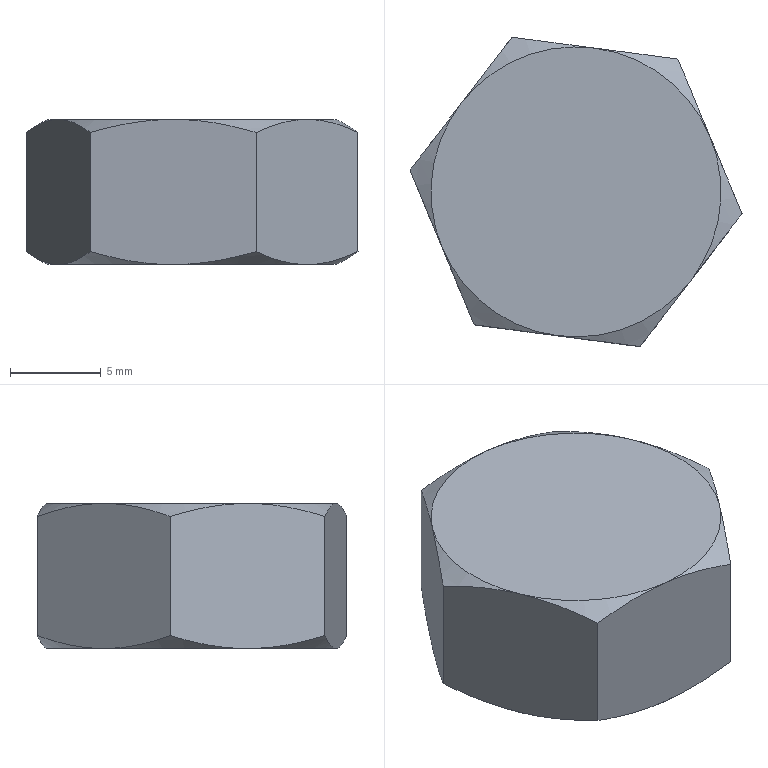Part | SolidWorks | features BaseBody 1 | 1 solid | 20 faces | box 18.318 x 17.066 x 8 mm | volume 1765 mm3 | cone 12 | plane 8
STEP:
#1=CARTESIAN_POINT('',(-45.504,-13.036,-254.55));
#2=VERTEX_POINT('',#1);
#3=CARTESIAN_POINT('',(-51.853,-8.168,-254.55));
#4=VERTEX_POINT('',#3);
#5=CARTESIAN_POINT('',(-44.463,-5.104,-254.55));
#6=DIRECTION('',(0.,0.,-1.));
#7=DIRECTION('',(-0.9237,-0.383,0.));
#8=AXIS2_PLACEMENT_3D('',#5,#6,#7);
#9=CIRCLE('',#8,8.);
#10=EDGE_CURVE('',#2,#4,#9,.T.);
#11=ORIENTED_EDGE('',*,*,#10,.T.);
#12=CARTESIAN_POINT('',(-50.812,-0.2362,-254.55));
#13=VERTEX_POINT('',#12);
#14=CARTESIAN_POINT('',(-44.463,-5.104,-254.55));
#15=DIRECTION('',(0.,0.,-1.));
#16=DIRECTION('',(-0.9237,-0.383,0.));
#17=AXIS2_PLACEMENT_3D('',#14,#15,#16);
#18=CIRCLE('',#17,8.);
#19=EDGE_CURVE('',#4,#13,#18,.T.);
#20=ORIENTED_EDGE('',*,*,#19,.T.);
#21=CARTESIAN_POINT('',(-43.422,2.828,-254.55));
#22=VERTEX_POINT('',#21);
#23=CARTESIAN_POINT('',(-44.463,-5.104,-254.55));
#24=DIRECTION('',(0.,0.,-1.));
#25=DIRECTION('',(-0.9237,-0.383,0.));
#26=AXIS2_PLACEMENT_3D('',#23,#24,#25);
#27=CIRCLE('',#26,8.);
#28=EDGE_CURVE('',#13,#22,#27,.T.);
#29=ORIENTED_EDGE('',*,*,#28,.T.);
#30=CARTESIAN_POINT('',(-37.073,-2.039,-254.55));
#31=VERTEX_POINT('',#30);
#32=CARTESIAN_POINT('',(-44.463,-5.104,-254.55));
#33=DIRECTION('',(0.,0.,1.));
#34=DIRECTION('',(0.9237,0.383,0.));
#35=AXIS2_PLACEMENT_3D('',#32,#33,#34);
#36=CIRCLE('',#35,8.);
#37=EDGE_CURVE('',#31,#22,#36,.T.);
#38=ORIENTED_EDGE('',*,*,#37,.F.);
#39=CARTESIAN_POINT('',(-38.114,-9.971,-254.55));
#40=VERTEX_POINT('',#39);
#41=CARTESIAN_POINT('',(-44.463,-5.104,-254.55));
#42=DIRECTION('',(0.,0.,-1.));
#43=DIRECTION('',(-0.9237,-0.383,0.));
#44=AXIS2_PLACEMENT_3D('',#41,#42,#43);
#45=CIRCLE('',#44,8.);
#46=EDGE_CURVE('',#31,#40,#45,.T.);
#47=ORIENTED_EDGE('',*,*,#46,.T.);
#48=CARTESIAN_POINT('',(-44.463,-5.104,-254.55));
#49=DIRECTION('',(0.,0.,-1.));
#50=DIRECTION('',(-0.9237,-0.383,0.));
#51=AXIS2_PLACEMENT_3D('',#48,#49,#50);
#52=CIRCLE('',#51,8.);
#53=EDGE_CURVE('',#40,#2,#52,.T.);
#54=ORIENTED_EDGE('',*,*,#53,.T.);
#55=EDGE_LOOP('',(#11,#20,#29,#38,#47,#54));
#56=FACE_OUTER_BOUND('',#55,.T.);
#57=CARTESIAN_POINT('',(-42.381,10.76,-254.55));
#58=DIRECTION('',(0.,0.,-1.));
#59=DIRECTION('',(0.,-1.,0.));
#60=AXIS2_PLACEMENT_3D('',#57,#58,#59);
#61=PLANE('',#60);
#62=ADVANCED_FACE('',(#56),#61,.T.);
#63=CARTESIAN_POINT('',(-53.622,-3.902,-253.835));
#64=VERTEX_POINT('',#63);
#65=CARTESIAN_POINT('',(-53.622,-3.902,-253.835));
#66=CARTESIAN_POINT('',(-53.163,-3.303,-254.053));
#67=CARTESIAN_POINT('',(-52.7,-2.699,-254.233));
#68=CARTESIAN_POINT('',(-51.764,-1.479,-254.482));
#69=CARTESIAN_POINT('',(-51.291,-0.8617,-254.55));
#70=CARTESIAN_POINT('',(-50.812,-0.2362,-254.55));
#71=B_SPLINE_CURVE_WITH_KNOTS('',3,(#65,#66,#67,#68,#69,#70),.UNSPECIFIED.,.F.,.F.,(4,2,4),(0.,0.002337,0.004674),.UNSPECIFIED.);
#72=EDGE_CURVE('',#64,#13,#71,.T.);
#73=ORIENTED_EDGE('',*,*,#72,.T.);
#74=ORIENTED_EDGE('',*,*,#19,.F.);
#75=CARTESIAN_POINT('',(-51.853,-8.168,-254.55));
#76=CARTESIAN_POINT('',(-52.155,-7.44,-254.55));
#77=CARTESIAN_POINT('',(-52.453,-6.722,-254.482));
#78=CARTESIAN_POINT('',(-53.042,-5.301,-254.233));
#79=CARTESIAN_POINT('',(-53.333,-4.599,-254.053));
#80=CARTESIAN_POINT('',(-53.622,-3.902,-253.835));
#81=B_SPLINE_CURVE_WITH_KNOTS('',3,(#75,#76,#77,#78,#79,#80),.UNSPECIFIED.,.F.,.F.,(4,2,4),(0.,0.002337,0.004674),.UNSPECIFIED.);
#82=EDGE_CURVE('',#4,#64,#81,.T.);
#83=ORIENTED_EDGE('',*,*,#82,.T.);
#84=EDGE_LOOP('',(#73,#74,#83));
#85=FACE_OUTER_BOUND('',#84,.T.);
#86=CARTESIAN_POINT('',(-44.463,-5.104,-251.646));
#87=DIRECTION('',(0.,0.,1.));
#88=DIRECTION('',(0.9237,0.383,0.));
#89=AXIS2_PLACEMENT_3D('',#86,#87,#88);
#90=CONICAL_SURFACE('',#89,13.029,1.047);
#91=ADVANCED_FACE('',(#85),#90,.T.);
#92=CARTESIAN_POINT('',(-48.001,3.429,-253.835));
#93=VERTEX_POINT('',#92);
#94=CARTESIAN_POINT('',(-50.812,-0.2362,-254.55));
#95=CARTESIAN_POINT('',(-50.332,0.3893,-254.55));
#96=CARTESIAN_POINT('',(-49.859,1.006,-254.482));
#97=CARTESIAN_POINT('',(-48.923,2.227,-254.233));
#98=CARTESIAN_POINT('',(-48.46,2.83,-254.053));
#99=CARTESIAN_POINT('',(-48.001,3.429,-253.835));
#100=B_SPLINE_CURVE_WITH_KNOTS('',3,(#94,#95,#96,#97,#98,#99),.UNSPECIFIED.,.F.,.F.,(4,2,4),(0.,0.002337,0.004674),.UNSPECIFIED.);
#101=EDGE_CURVE('',#13,#93,#100,.T.);
#102=ORIENTED_EDGE('',*,*,#101,.T.);
#103=CARTESIAN_POINT('',(-48.001,3.429,-253.835));
#104=CARTESIAN_POINT('',(-47.253,3.331,-254.053));
#105=CARTESIAN_POINT('',(-46.499,3.232,-254.233));
#106=CARTESIAN_POINT('',(-44.974,3.032,-254.482));
#107=CARTESIAN_POINT('',(-44.203,2.931,-254.55));
#108=CARTESIAN_POINT('',(-43.422,2.828,-254.55));
#109=B_SPLINE_CURVE_WITH_KNOTS('',3,(#103,#104,#105,#106,#107,#108),.UNSPECIFIED.,.F.,.F.,(4,2,4),(0.,0.002337,0.004674),.UNSPECIFIED.);
#110=EDGE_CURVE('',#93,#22,#109,.T.);
#111=ORIENTED_EDGE('',*,*,#110,.T.);
#112=ORIENTED_EDGE('',*,*,#28,.F.);
#113=EDGE_LOOP('',(#102,#111,#112));
#114=FACE_OUTER_BOUND('',#113,.T.);
#115=CARTESIAN_POINT('',(-44.463,-5.104,-251.646));
#116=DIRECTION('',(0.,0.,1.));
#117=DIRECTION('',(0.9237,0.383,0.));
#118=AXIS2_PLACEMENT_3D('',#115,#116,#117);
#119=CONICAL_SURFACE('',#118,13.029,1.047);
#120=ADVANCED_FACE('',(#114),#119,.T.);
#121=CARTESIAN_POINT('',(-38.842,2.227,-253.835));
#122=VERTEX_POINT('',#121);
#123=CARTESIAN_POINT('',(-43.422,2.828,-254.55));
#124=CARTESIAN_POINT('',(-42.64,2.726,-254.55));
#125=CARTESIAN_POINT('',(-41.869,2.624,-254.482));
#126=CARTESIAN_POINT('',(-40.344,2.424,-254.233));
#127=CARTESIAN_POINT('',(-39.59,2.325,-254.053));
#128=CARTESIAN_POINT('',(-38.842,2.227,-253.835));
#129=B_SPLINE_CURVE_WITH_KNOTS('',3,(#123,#124,#125,#126,#127,#128),.UNSPECIFIED.,.F.,.F.,(4,2,4),(0.,0.002337,0.004674),.UNSPECIFIED.);
#130=EDGE_CURVE('',#22,#122,#129,.T.);
#131=ORIENTED_EDGE('',*,*,#130,.T.);
#132=CARTESIAN_POINT('',(-38.842,2.227,-253.835));
#133=CARTESIAN_POINT('',(-38.553,1.53,-254.053));
#134=CARTESIAN_POINT('',(-38.262,0.8277,-254.233));
#135=CARTESIAN_POINT('',(-37.673,-0.5929,-254.482));
#136=CARTESIAN_POINT('',(-37.375,-1.311,-254.55));
#137=CARTESIAN_POINT('',(-37.073,-2.039,-254.55));
#138=B_SPLINE_CURVE_WITH_KNOTS('',3,(#132,#133,#134,#135,#136,#137),.UNSPECIFIED.,.F.,.F.,(4,2,4),(0.,0.002337,0.004674),.UNSPECIFIED.);
#139=EDGE_CURVE('',#122,#31,#138,.T.);
#140=ORIENTED_EDGE('',*,*,#139,.T.);
#141=ORIENTED_EDGE('',*,*,#37,.T.);
#142=EDGE_LOOP('',(#131,#140,#141));
#143=FACE_OUTER_BOUND('',#142,.T.);
#144=CARTESIAN_POINT('',(-44.463,-5.104,-251.646));
#145=DIRECTION('',(0.,0.,1.));
#146=DIRECTION('',(0.9237,0.383,0.));
#147=AXIS2_PLACEMENT_3D('',#144,#145,#146);
#148=CONICAL_SURFACE('',#147,13.029,1.047);
#149=ADVANCED_FACE('',(#143),#148,.T.);
#150=CARTESIAN_POINT('',(-35.304,-6.306,-253.835));
#151=VERTEX_POINT('',#150);
#152=CARTESIAN_POINT('',(-37.073,-2.039,-254.55));
#153=CARTESIAN_POINT('',(-36.771,-2.767,-254.55));
#154=CARTESIAN_POINT('',(-36.473,-3.486,-254.482));
#155=CARTESIAN_POINT('',(-35.884,-4.906,-254.233));
#156=CARTESIAN_POINT('',(-35.593,-5.609,-254.053));
#157=CARTESIAN_POINT('',(-35.304,-6.306,-253.835));
#158=B_SPLINE_CURVE_WITH_KNOTS('',3,(#152,#153,#154,#155,#156,#157),.UNSPECIFIED.,.F.,.F.,(4,2,4),(0.,0.002337,0.004674),.UNSPECIFIED.);
#159=EDGE_CURVE('',#31,#151,#158,.T.);
#160=ORIENTED_EDGE('',*,*,#159,.T.);
#161=CARTESIAN_POINT('',(-35.304,-6.306,-253.835));
#162=CARTESIAN_POINT('',(-35.763,-6.905,-254.053));
#163=CARTESIAN_POINT('',(-36.226,-7.508,-254.233));
#164=CARTESIAN_POINT('',(-37.161,-8.729,-254.482));
#165=CARTESIAN_POINT('',(-37.635,-9.346,-254.55));
#166=CARTESIAN_POINT('',(-38.114,-9.971,-254.55));
#167=B_SPLINE_CURVE_WITH_KNOTS('',3,(#161,#162,#163,#164,#165,#166),.UNSPECIFIED.,.F.,.F.,(4,2,4),(0.,0.002337,0.004674),.UNSPECIFIED.);
#168=EDGE_CURVE('',#151,#40,#167,.T.);
#169=ORIENTED_EDGE('',*,*,#168,.T.);
#170=ORIENTED_EDGE('',*,*,#46,.F.);
#171=EDGE_LOOP('',(#160,#169,#170));
#172=FACE_OUTER_BOUND('',#171,.T.);
#173=CARTESIAN_POINT('',(-44.463,-5.104,-251.646));
#174=DIRECTION('',(0.,0.,1.));
#175=DIRECTION('',(0.9237,0.383,0.));
#176=AXIS2_PLACEMENT_3D('',#173,#174,#175);
#177=CONICAL_SURFACE('',#176,13.029,1.047);
#178=ADVANCED_FACE('',(#172),#177,.T.);
#179=CARTESIAN_POINT('',(-40.924,-13.637,-253.835));
#180=VERTEX_POINT('',#179);
#181=CARTESIAN_POINT('',(-38.114,-9.971,-254.55));
#182=CARTESIAN_POINT('',(-38.594,-10.597,-254.55));
#183=CARTESIAN_POINT('',(-39.067,-11.214,-254.482));
#184=CARTESIAN_POINT('',(-40.003,-12.435,-254.233));
#185=CARTESIAN_POINT('',(-40.465,-13.038,-254.053));
#186=CARTESIAN_POINT('',(-40.924,-13.637,-253.835));
#187=B_SPLINE_CURVE_WITH_KNOTS('',3,(#181,#182,#183,#184,#185,#186),.UNSPECIFIED.,.F.,.F.,(4,2,4),(0.,0.002337,0.004674),.UNSPECIFIED.);
#188=EDGE_CURVE('',#40,#180,#187,.T.);
#189=ORIENTED_EDGE('',*,*,#188,.T.);
#190=CARTESIAN_POINT('',(-40.924,-13.637,-253.835));
#191=CARTESIAN_POINT('',(-41.673,-13.539,-254.053));
#192=CARTESIAN_POINT('',(-42.426,-13.44,-254.233));
#193=CARTESIAN_POINT('',(-43.951,-13.24,-254.482));
#194=CARTESIAN_POINT('',(-44.722,-13.138,-254.55));
#195=CARTESIAN_POINT('',(-45.504,-13.036,-254.55));
#196=B_SPLINE_CURVE_WITH_KNOTS('',3,(#190,#191,#192,#193,#194,#195),.UNSPECIFIED.,.F.,.F.,(4,2,4),(0.,0.002337,0.004674),.UNSPECIFIED.);
#197=EDGE_CURVE('',#180,#2,#196,.T.);
#198=ORIENTED_EDGE('',*,*,#197,.T.);
#199=ORIENTED_EDGE('',*,*,#53,.F.);
#200=EDGE_LOOP('',(#189,#198,#199));
#201=FACE_OUTER_BOUND('',#200,.T.);
#202=CARTESIAN_POINT('',(-44.463,-5.104,-251.646));
#203=DIRECTION('',(0.,0.,1.));
#204=DIRECTION('',(0.9237,0.383,0.));
#205=AXIS2_PLACEMENT_3D('',#202,#203,#204);
#206=CONICAL_SURFACE('',#205,13.029,1.047);
#207=ADVANCED_FACE('',(#201),#206,.T.);
#208=CARTESIAN_POINT('',(-50.083,-12.435,-253.835));
#209=VERTEX_POINT('',#208);
#210=CARTESIAN_POINT('',(-45.504,-13.036,-254.55));
#211=CARTESIAN_POINT('',(-46.285,-12.933,-254.55));
#212=CARTESIAN_POINT('',(-47.057,-12.832,-254.482));
#213=CARTESIAN_POINT('',(-48.581,-12.632,-254.233));
#214=CARTESIAN_POINT('',(-49.335,-12.533,-254.053));
#215=CARTESIAN_POINT('',(-50.083,-12.435,-253.835));
#216=B_SPLINE_CURVE_WITH_KNOTS('',3,(#210,#211,#212,#213,#214,#215),.UNSPECIFIED.,.F.,.F.,(4,2,4),(0.,0.002337,0.004674),.UNSPECIFIED.);
#217=EDGE_CURVE('',#2,#209,#216,.T.);
#218=ORIENTED_EDGE('',*,*,#217,.T.);
#219=CARTESIAN_POINT('',(-50.083,-12.435,-253.835));
#220=CARTESIAN_POINT('',(-50.372,-11.738,-254.053));
#221=CARTESIAN_POINT('',(-50.664,-11.035,-254.233));
#222=CARTESIAN_POINT('',(-51.253,-9.615,-254.482));
#223=CARTESIAN_POINT('',(-51.551,-8.896,-254.55));
#224=CARTESIAN_POINT('',(-51.853,-8.168,-254.55));
#225=B_SPLINE_CURVE_WITH_KNOTS('',3,(#219,#220,#221,#222,#223,#224),.UNSPECIFIED.,.F.,.F.,(4,2,4),(0.,0.002337,0.004674),.UNSPECIFIED.);
#226=EDGE_CURVE('',#209,#4,#225,.T.);
#227=ORIENTED_EDGE('',*,*,#226,.T.);
#228=ORIENTED_EDGE('',*,*,#10,.F.);
#229=EDGE_LOOP('',(#218,#227,#228));
#230=FACE_OUTER_BOUND('',#229,.T.);
#231=CARTESIAN_POINT('',(-44.463,-5.104,-251.646));
#232=DIRECTION('',(0.,0.,1.));
#233=DIRECTION('',(0.9237,0.383,0.));
#234=AXIS2_PLACEMENT_3D('',#231,#232,#233);
#235=CONICAL_SURFACE('',#234,13.029,1.047);
#236=ADVANCED_FACE('',(#230),#235,.T.);
#237=CARTESIAN_POINT('',(-51.853,-8.168,-246.55));
#238=VERTEX_POINT('',#237);
#239=CARTESIAN_POINT('',(-50.812,-0.2362,-246.55));
#240=VERTEX_POINT('',#239);
#241=CARTESIAN_POINT('',(-44.463,-5.104,-246.55));
#242=DIRECTION('',(0.,0.,-1.));
#243=DIRECTION('',(-0.9237,-0.383,0.));
#244=AXIS2_PLACEMENT_3D('',#241,#242,#243);
#245=CIRCLE('',#244,8.);
#246=EDGE_CURVE('',#238,#240,#245,.T.);
#247=ORIENTED_EDGE('',*,*,#246,.F.);
#248=CARTESIAN_POINT('',(-45.504,-13.036,-246.55));
#249=VERTEX_POINT('',#248);
#250=CARTESIAN_POINT('',(-44.463,-5.104,-246.55));
#251=DIRECTION('',(0.,0.,-1.));
#252=DIRECTION('',(-0.9237,-0.383,0.));
#253=AXIS2_PLACEMENT_3D('',#250,#251,#252);
#254=CIRCLE('',#253,8.);
#255=EDGE_CURVE('',#249,#238,#254,.T.);
#256=ORIENTED_EDGE('',*,*,#255,.F.);
#257=CARTESIAN_POINT('',(-38.114,-9.971,-246.55));
#258=VERTEX_POINT('',#257);
#259=CARTESIAN_POINT('',(-44.463,-5.104,-246.55));
#260=DIRECTION('',(0.,0.,-1.));
#261=DIRECTION('',(-0.9237,-0.383,0.));
#262=AXIS2_PLACEMENT_3D('',#259,#260,#261);
#263=CIRCLE('',#262,8.);
#264=EDGE_CURVE('',#258,#249,#263,.T.);
#265=ORIENTED_EDGE('',*,*,#264,.F.);
#266=CARTESIAN_POINT('',(-37.073,-2.039,-246.55));
#267=VERTEX_POINT('',#266);
#268=CARTESIAN_POINT('',(-44.463,-5.104,-246.55));
#269=DIRECTION('',(0.,0.,-1.));
#270=DIRECTION('',(-0.9237,-0.383,0.));
#271=AXIS2_PLACEMENT_3D('',#268,#269,#270);
#272=CIRCLE('',#271,8.);
#273=EDGE_CURVE('',#267,#258,#272,.T.);
#274=ORIENTED_EDGE('',*,*,#273,.F.);
#275=CARTESIAN_POINT('',(-43.422,2.828,-246.55));
#276=VERTEX_POINT('',#275);
#277=CARTESIAN_POINT('',(-44.463,-5.104,-246.55));
#278=DIRECTION('',(0.,0.,1.));
#279=DIRECTION('',(0.9237,0.383,0.));
#280=AXIS2_PLACEMENT_3D('',#277,#278,#279);
#281=CIRCLE('',#280,8.);
#282=EDGE_CURVE('',#267,#276,#281,.T.);
#283=ORIENTED_EDGE('',*,*,#282,.T.);
#284=CARTESIAN_POINT('',(-44.463,-5.104,-246.55));
#285=DIRECTION('',(0.,0.,-1.));
#286=DIRECTION('',(-0.9237,-0.383,0.));
#287=AXIS2_PLACEMENT_3D('',#284,#285,#286);
#288=CIRCLE('',#287,8.);
#289=EDGE_CURVE('',#240,#276,#288,.T.);
#290=ORIENTED_EDGE('',*,*,#289,.F.);
#291=EDGE_LOOP('',(#247,#256,#265,#274,#283,#290));
#292=FACE_OUTER_BOUND('',#291,.T.);
#293=CARTESIAN_POINT('',(-42.381,10.76,-246.55));
#294=DIRECTION('',(0.,0.,-1.));
#295=DIRECTION('',(0.,-1.,0.));
#296=AXIS2_PLACEMENT_3D('',#293,#294,#295);
#297=PLANE('',#296);
#298=ADVANCED_FACE('',(#292),#297,.F.);
#299=CARTESIAN_POINT('',(-53.622,-3.902,-247.265));
#300=VERTEX_POINT('',#299);
#301=CARTESIAN_POINT('',(-50.812,-0.2362,-246.55));
#302=CARTESIAN_POINT('',(-51.291,-0.8617,-246.55));
#303=CARTESIAN_POINT('',(-51.764,-1.479,-246.618));
#304=CARTESIAN_POINT('',(-52.7,-2.699,-246.867));
#305=CARTESIAN_POINT('',(-53.163,-3.303,-247.047));
#306=CARTESIAN_POINT('',(-53.622,-3.902,-247.265));
#307=B_SPLINE_CURVE_WITH_KNOTS('',3,(#301,#302,#303,#304,#305,#306),.UNSPECIFIED.,.F.,.F.,(4,2,4),(0.,0.002337,0.004674),.UNSPECIFIED.);
#308=EDGE_CURVE('',#240,#300,#307,.T.);
#309=ORIENTED_EDGE('',*,*,#308,.T.);
#310=CARTESIAN_POINT('',(-53.622,-3.902,-247.265));
#311=CARTESIAN_POINT('',(-53.333,-4.599,-247.047));
#312=CARTESIAN_POINT('',(-53.042,-5.301,-246.867));
#313=CARTESIAN_POINT('',(-52.453,-6.722,-246.618));
#314=CARTESIAN_POINT('',(-52.155,-7.44,-246.55));
#315=CARTESIAN_POINT('',(-51.853,-8.168,-246.55));
#316=B_SPLINE_CURVE_WITH_KNOTS('',3,(#310,#311,#312,#313,#314,#315),.UNSPECIFIED.,.F.,.F.,(4,2,4),(0.,0.002337,0.004674),.UNSPECIFIED.);
#317=EDGE_CURVE('',#300,#238,#316,.T.);
#318=ORIENTED_EDGE('',*,*,#317,.T.);
#319=ORIENTED_EDGE('',*,*,#246,.T.);
#320=EDGE_LOOP('',(#309,#318,#319));
#321=FACE_OUTER_BOUND('',#320,.T.);
#322=CARTESIAN_POINT('',(-44.463,-5.104,-246.55));
#323=DIRECTION('',(0.,0.,-1.));
#324=DIRECTION('',(-0.9237,-0.383,0.));
#325=AXIS2_PLACEMENT_3D('',#322,#323,#324);
#326=CONICAL_SURFACE('',#325,8.,1.047);
#327=ADVANCED_FACE('',(#321),#326,.T.);
#328=CARTESIAN_POINT('',(-48.001,3.429,-247.265));
#329=VERTEX_POINT('',#328);
#330=CARTESIAN_POINT('',(-43.422,2.828,-246.55));
#331=CARTESIAN_POINT('',(-44.203,2.931,-246.55));
#332=CARTESIAN_POINT('',(-44.974,3.032,-246.618));
#333=CARTESIAN_POINT('',(-46.499,3.232,-246.867));
#334=CARTESIAN_POINT('',(-47.253,3.331,-247.047));
#335=CARTESIAN_POINT('',(-48.001,3.429,-247.265));
#336=B_SPLINE_CURVE_WITH_KNOTS('',3,(#330,#331,#332,#333,#334,#335),.UNSPECIFIED.,.F.,.F.,(4,2,4),(0.,0.002337,0.004674),.UNSPECIFIED.);
#337=EDGE_CURVE('',#276,#329,#336,.T.);
#338=ORIENTED_EDGE('',*,*,#337,.T.);
#339=CARTESIAN_POINT('',(-48.001,3.429,-247.265));
#340=CARTESIAN_POINT('',(-48.46,2.83,-247.047));
#341=CARTESIAN_POINT('',(-48.923,2.227,-246.867));
#342=CARTESIAN_POINT('',(-49.859,1.006,-246.618));
#343=CARTESIAN_POINT('',(-50.332,0.3893,-246.55));
#344=CARTESIAN_POINT('',(-50.812,-0.2362,-246.55));
#345=B_SPLINE_CURVE_WITH_KNOTS('',3,(#339,#340,#341,#342,#343,#344),.UNSPECIFIED.,.F.,.F.,(4,2,4),(0.,0.002337,0.004674),.UNSPECIFIED.);
#346=EDGE_CURVE('',#329,#240,#345,.T.);
#347=ORIENTED_EDGE('',*,*,#346,.T.);
#348=ORIENTED_EDGE('',*,*,#289,.T.);
#349=EDGE_LOOP('',(#338,#347,#348));
#350=FACE_OUTER_BOUND('',#349,.T.);
#351=CARTESIAN_POINT('',(-44.463,-5.104,-246.55));
#352=DIRECTION('',(0.,0.,-1.));
#353=DIRECTION('',(-0.9237,-0.383,0.));
#354=AXIS2_PLACEMENT_3D('',#351,#352,#353);
#355=CONICAL_SURFACE('',#354,8.,1.047);
#356=ADVANCED_FACE('',(#350),#355,.T.);
#357=CARTESIAN_POINT('',(-38.842,2.227,-247.265));
#358=VERTEX_POINT('',#357);
#359=CARTESIAN_POINT('',(-37.073,-2.039,-246.55));
#360=CARTESIAN_POINT('',(-37.375,-1.311,-246.55));
#361=CARTESIAN_POINT('',(-37.673,-0.5929,-246.618));
#362=CARTESIAN_POINT('',(-38.262,0.8277,-246.867));
#363=CARTESIAN_POINT('',(-38.553,1.53,-247.047));
#364=CARTESIAN_POINT('',(-38.842,2.227,-247.265));
#365=B_SPLINE_CURVE_WITH_KNOTS('',3,(#359,#360,#361,#362,#363,#364),.UNSPECIFIED.,.F.,.F.,(4,2,4),(0.,0.002337,0.004674),.UNSPECIFIED.);
#366=EDGE_CURVE('',#267,#358,#365,.T.);
#367=ORIENTED_EDGE('',*,*,#366,.T.);
#368=CARTESIAN_POINT('',(-38.842,2.227,-247.265));
#369=CARTESIAN_POINT('',(-39.59,2.325,-247.047));
#370=CARTESIAN_POINT('',(-40.344,2.424,-246.867));
#371=CARTESIAN_POINT('',(-41.869,2.624,-246.618));
#372=CARTESIAN_POINT('',(-42.64,2.726,-246.55));
#373=CARTESIAN_POINT('',(-43.422,2.828,-246.55));
#374=B_SPLINE_CURVE_WITH_KNOTS('',3,(#368,#369,#370,#371,#372,#373),.UNSPECIFIED.,.F.,.F.,(4,2,4),(0.,0.002337,0.004674),.UNSPECIFIED.);
#375=EDGE_CURVE('',#358,#276,#374,.T.);
#376=ORIENTED_EDGE('',*,*,#375,.T.);
#377=ORIENTED_EDGE('',*,*,#282,.F.);
#378=EDGE_LOOP('',(#367,#376,#377));
#379=FACE_OUTER_BOUND('',#378,.T.);
#380=CARTESIAN_POINT('',(-44.463,-5.104,-246.55));
#381=DIRECTION('',(0.,0.,-1.));
#382=DIRECTION('',(-0.9237,-0.383,0.));
#383=AXIS2_PLACEMENT_3D('',#380,#381,#382);
#384=CONICAL_SURFACE('',#383,8.,1.047);
#385=ADVANCED_FACE('',(#379),#384,.T.);
#386=CARTESIAN_POINT('',(-35.304,-6.306,-247.265));
#387=VERTEX_POINT('',#386);
#388=CARTESIAN_POINT('',(-35.304,-6.306,-247.265));
#389=CARTESIAN_POINT('',(-35.593,-5.609,-247.047));
#390=CARTESIAN_POINT('',(-35.884,-4.906,-246.867));
#391=CARTESIAN_POINT('',(-36.473,-3.486,-246.618));
#392=CARTESIAN_POINT('',(-36.771,-2.767,-246.55));
#393=CARTESIAN_POINT('',(-37.073,-2.039,-246.55));
#394=B_SPLINE_CURVE_WITH_KNOTS('',3,(#388,#389,#390,#391,#392,#393),.UNSPECIFIED.,.F.,.F.,(4,2,4),(0.,0.002337,0.004674),.UNSPECIFIED.);
#395=EDGE_CURVE('',#387,#267,#394,.T.);
#396=ORIENTED_EDGE('',*,*,#395,.T.);
#397=ORIENTED_EDGE('',*,*,#273,.T.);
#398=CARTESIAN_POINT('',(-38.114,-9.971,-246.55));
#399=CARTESIAN_POINT('',(-37.635,-9.346,-246.55));
#400=CARTESIAN_POINT('',(-37.161,-8.729,-246.618));
#401=CARTESIAN_POINT('',(-36.226,-7.508,-246.867));
#402=CARTESIAN_POINT('',(-35.763,-6.905,-247.047));
#403=CARTESIAN_POINT('',(-35.304,-6.306,-247.265));
#404=B_SPLINE_CURVE_WITH_KNOTS('',3,(#398,#399,#400,#401,#402,#403),.UNSPECIFIED.,.F.,.F.,(4,2,4),(0.,0.002337,0.004674),.UNSPECIFIED.);
#405=EDGE_CURVE('',#258,#387,#404,.T.);
#406=ORIENTED_EDGE('',*,*,#405,.T.);
#407=EDGE_LOOP('',(#396,#397,#406));
#408=FACE_OUTER_BOUND('',#407,.T.);
#409=CARTESIAN_POINT('',(-44.463,-5.104,-246.55));
#410=DIRECTION('',(0.,0.,-1.));
#411=DIRECTION('',(-0.9237,-0.383,0.));
#412=AXIS2_PLACEMENT_3D('',#409,#410,#411);
#413=CONICAL_SURFACE('',#412,8.,1.047);
#414=ADVANCED_FACE('',(#408),#413,.T.);
#415=CARTESIAN_POINT('',(-40.924,-13.637,-247.265));
#416=VERTEX_POINT('',#415);
#417=CARTESIAN_POINT('',(-40.924,-13.637,-247.265));
#418=CARTESIAN_POINT('',(-40.465,-13.038,-247.047));
#419=CARTESIAN_POINT('',(-40.003,-12.435,-246.867));
#420=CARTESIAN_POINT('',(-39.067,-11.214,-246.618));
#421=CARTESIAN_POINT('',(-38.594,-10.597,-246.55));
#422=CARTESIAN_POINT('',(-38.114,-9.971,-246.55));
#423=B_SPLINE_CURVE_WITH_KNOTS('',3,(#417,#418,#419,#420,#421,#422),.UNSPECIFIED.,.F.,.F.,(4,2,4),(0.,0.002337,0.004674),.UNSPECIFIED.);
#424=EDGE_CURVE('',#416,#258,#423,.T.);
#425=ORIENTED_EDGE('',*,*,#424,.T.);
#426=ORIENTED_EDGE('',*,*,#264,.T.);
#427=CARTESIAN_POINT('',(-45.504,-13.036,-246.55));
#428=CARTESIAN_POINT('',(-44.722,-13.138,-246.55));
#429=CARTESIAN_POINT('',(-43.951,-13.24,-246.618));
#430=CARTESIAN_POINT('',(-42.426,-13.44,-246.867));
#431=CARTESIAN_POINT('',(-41.673,-13.539,-247.047));
#432=CARTESIAN_POINT('',(-40.924,-13.637,-247.265));
#433=B_SPLINE_CURVE_WITH_KNOTS('',3,(#427,#428,#429,#430,#431,#432),.UNSPECIFIED.,.F.,.F.,(4,2,4),(0.,0.002337,0.004674),.UNSPECIFIED.);
#434=EDGE_CURVE('',#249,#416,#433,.T.);
#435=ORIENTED_EDGE('',*,*,#434,.T.);
#436=EDGE_LOOP('',(#425,#426,#435));
#437=FACE_OUTER_BOUND('',#436,.T.);
#438=CARTESIAN_POINT('',(-44.463,-5.104,-246.55));
#439=DIRECTION('',(0.,0.,-1.));
#440=DIRECTION('',(-0.9237,-0.383,0.));
#441=AXIS2_PLACEMENT_3D('',#438,#439,#440);
#442=CONICAL_SURFACE('',#441,8.,1.047);
#443=ADVANCED_FACE('',(#437),#442,.T.);
#444=CARTESIAN_POINT('',(-50.083,-12.435,-247.265));
#445=VERTEX_POINT('',#444);
#446=CARTESIAN_POINT('',(-50.083,-12.435,-247.265));
#447=CARTESIAN_POINT('',(-49.335,-12.533,-247.047));
#448=CARTESIAN_POINT('',(-48.581,-12.632,-246.867));
#449=CARTESIAN_POINT('',(-47.057,-12.832,-246.618));
#450=CARTESIAN_POINT('',(-46.285,-12.933,-246.55));
#451=CARTESIAN_POINT('',(-45.504,-13.036,-246.55));
#452=B_SPLINE_CURVE_WITH_KNOTS('',3,(#446,#447,#448,#449,#450,#451),.UNSPECIFIED.,.F.,.F.,(4,2,4),(0.,0.002337,0.004674),.UNSPECIFIED.);
#453=EDGE_CURVE('',#445,#249,#452,.T.);
#454=ORIENTED_EDGE('',*,*,#453,.T.);
#455=ORIENTED_EDGE('',*,*,#255,.T.);
#456=CARTESIAN_POINT('',(-51.853,-8.168,-246.55));
#457=CARTESIAN_POINT('',(-51.551,-8.896,-246.55));
#458=CARTESIAN_POINT('',(-51.253,-9.615,-246.618));
#459=CARTESIAN_POINT('',(-50.664,-11.035,-246.867));
#460=CARTESIAN_POINT('',(-50.372,-11.738,-247.047));
#461=CARTESIAN_POINT('',(-50.083,-12.435,-247.265));
#462=B_SPLINE_CURVE_WITH_KNOTS('',3,(#456,#457,#458,#459,#460,#461),.UNSPECIFIED.,.F.,.F.,(4,2,4),(0.,0.002337,0.004674),.UNSPECIFIED.);
#463=EDGE_CURVE('',#238,#445,#462,.T.);
#464=ORIENTED_EDGE('',*,*,#463,.T.);
#465=EDGE_LOOP('',(#454,#455,#464));
#466=FACE_OUTER_BOUND('',#465,.T.);
#467=CARTESIAN_POINT('',(-44.463,-5.104,-246.55));
#468=DIRECTION('',(0.,0.,-1.));
#469=DIRECTION('',(-0.9237,-0.383,0.));
#470=AXIS2_PLACEMENT_3D('',#467,#468,#469);
#471=CONICAL_SURFACE('',#470,8.,1.047);
#472=ADVANCED_FACE('',(#466),#471,.T.);
#473=ORIENTED_EDGE('',*,*,#226,.F.);
#474=CARTESIAN_POINT('',(-50.083,-12.435,-254.55));
#475=DIRECTION('',(0.,0.,1.));
#476=VECTOR('',#475,1000.);
#477=LINE('',#474,#476);
#478=EDGE_CURVE('',#209,#445,#477,.T.);
#479=ORIENTED_EDGE('',*,*,#478,.T.);
#480=ORIENTED_EDGE('',*,*,#463,.F.);
#481=ORIENTED_EDGE('',*,*,#317,.F.);
#482=CARTESIAN_POINT('',(-53.622,-3.902,-254.55));
#483=DIRECTION('',(0.,0.,1.));
#484=VECTOR('',#483,1000.);
#485=LINE('',#482,#484);
#486=EDGE_CURVE('',#64,#300,#485,.T.);
#487=ORIENTED_EDGE('',*,*,#486,.F.);
#488=ORIENTED_EDGE('',*,*,#82,.F.);
#489=EDGE_LOOP('',(#473,#479,#480,#481,#487,#488));
#490=FACE_OUTER_BOUND('',#489,.T.);
#491=CARTESIAN_POINT('',(-50.083,-12.435,-254.55));
#492=DIRECTION('',(0.9237,0.383,0.));
#493=DIRECTION('',(0.,0.,-1.));
#494=AXIS2_PLACEMENT_3D('',#491,#492,#493);
#495=PLANE('',#494);
#496=ADVANCED_FACE('',(#490),#495,.F.);
#497=ORIENTED_EDGE('',*,*,#197,.F.);
#498=CARTESIAN_POINT('',(-40.924,-13.637,-254.55));
#499=DIRECTION('',(0.,0.,1.));
#500=VECTOR('',#499,1000.);
#501=LINE('',#498,#500);
#502=EDGE_CURVE('',#180,#416,#501,.T.);
#503=ORIENTED_EDGE('',*,*,#502,.T.);
#504=ORIENTED_EDGE('',*,*,#434,.F.);
#505=ORIENTED_EDGE('',*,*,#453,.F.);
#506=ORIENTED_EDGE('',*,*,#478,.F.);
#507=ORIENTED_EDGE('',*,*,#217,.F.);
#508=EDGE_LOOP('',(#497,#503,#504,#505,#506,#507));
#509=FACE_OUTER_BOUND('',#508,.T.);
#510=CARTESIAN_POINT('',(-40.924,-13.637,-254.55));
#511=DIRECTION('',(0.1301,0.9915,0.));
#512=DIRECTION('',(0.,0.,-1.));
#513=AXIS2_PLACEMENT_3D('',#510,#511,#512);
#514=PLANE('',#513);
#515=ADVANCED_FACE('',(#509),#514,.F.);
#516=ORIENTED_EDGE('',*,*,#168,.F.);
#517=CARTESIAN_POINT('',(-35.304,-6.306,-254.55));
#518=DIRECTION('',(0.,0.,1.));
#519=VECTOR('',#518,1000.);
#520=LINE('',#517,#519);
#521=EDGE_CURVE('',#151,#387,#520,.T.);
#522=ORIENTED_EDGE('',*,*,#521,.T.);
#523=ORIENTED_EDGE('',*,*,#405,.F.);
#524=ORIENTED_EDGE('',*,*,#424,.F.);
#525=ORIENTED_EDGE('',*,*,#502,.F.);
#526=ORIENTED_EDGE('',*,*,#188,.F.);
#527=EDGE_LOOP('',(#516,#522,#523,#524,#525,#526));
#528=FACE_OUTER_BOUND('',#527,.T.);
#529=CARTESIAN_POINT('',(-35.304,-6.306,-254.55));
#530=DIRECTION('',(-0.7936,0.6084,0.));
#531=DIRECTION('',(0.,0.,1.));
#532=AXIS2_PLACEMENT_3D('',#529,#530,#531);
#533=PLANE('',#532);
#534=ADVANCED_FACE('',(#528),#533,.F.);
#535=ORIENTED_EDGE('',*,*,#139,.F.);
#536=CARTESIAN_POINT('',(-38.842,2.227,-254.55));
#537=DIRECTION('',(0.,0.,1.));
#538=VECTOR('',#537,1000.);
#539=LINE('',#536,#538);
#540=EDGE_CURVE('',#122,#358,#539,.T.);
#541=ORIENTED_EDGE('',*,*,#540,.T.);
#542=ORIENTED_EDGE('',*,*,#366,.F.);
#543=ORIENTED_EDGE('',*,*,#395,.F.);
#544=ORIENTED_EDGE('',*,*,#521,.F.);
#545=ORIENTED_EDGE('',*,*,#159,.F.);
#546=EDGE_LOOP('',(#535,#541,#542,#543,#544,#545));
#547=FACE_OUTER_BOUND('',#546,.T.);
#548=CARTESIAN_POINT('',(-38.842,2.227,-254.55));
#549=DIRECTION('',(-0.9237,-0.383,0.));
#550=DIRECTION('',(-0.383,0.9237,0.));
#551=AXIS2_PLACEMENT_3D('',#548,#549,#550);
#552=PLANE('',#551);
#553=ADVANCED_FACE('',(#547),#552,.F.);
#554=ORIENTED_EDGE('',*,*,#110,.F.);
#555=CARTESIAN_POINT('',(-48.001,3.429,-254.55));
#556=DIRECTION('',(0.,0.,1.));
#557=VECTOR('',#556,1000.);
#558=LINE('',#555,#557);
#559=EDGE_CURVE('',#93,#329,#558,.T.);
#560=ORIENTED_EDGE('',*,*,#559,.T.);
#561=ORIENTED_EDGE('',*,*,#337,.F.);
#562=ORIENTED_EDGE('',*,*,#375,.F.);
#563=ORIENTED_EDGE('',*,*,#540,.F.);
#564=ORIENTED_EDGE('',*,*,#130,.F.);
#565=EDGE_LOOP('',(#554,#560,#561,#562,#563,#564));
#566=FACE_OUTER_BOUND('',#565,.T.);
#567=CARTESIAN_POINT('',(-48.001,3.429,-254.55));
#568=DIRECTION('',(-0.1301,-0.9915,0.));
#569=DIRECTION('',(-0.9915,0.1301,0.));
#570=AXIS2_PLACEMENT_3D('',#567,#568,#569);
#571=PLANE('',#570);
#572=ADVANCED_FACE('',(#566),#571,.F.);
#573=ORIENTED_EDGE('',*,*,#72,.F.);
#574=ORIENTED_EDGE('',*,*,#486,.T.);
#575=ORIENTED_EDGE('',*,*,#308,.F.);
#576=ORIENTED_EDGE('',*,*,#346,.F.);
#577=ORIENTED_EDGE('',*,*,#559,.F.);
#578=ORIENTED_EDGE('',*,*,#101,.F.);
#579=EDGE_LOOP('',(#573,#574,#575,#576,#577,#578));
#580=FACE_OUTER_BOUND('',#579,.T.);
#581=CARTESIAN_POINT('',(-53.622,-3.902,-254.55));
#582=DIRECTION('',(0.7936,-0.6084,0.));
#583=DIRECTION('',(0.,0.,-1.));
#584=AXIS2_PLACEMENT_3D('',#581,#582,#583);
#585=PLANE('',#584);
#586=ADVANCED_FACE('',(#580),#585,.F.);
#587=CLOSED_SHELL('',(#62,#91,#120,#149,#178,#207,#236,#298,#327,#356,#385,#414,#443,#472,#496,#515,#534,#553,#572,#586));
#588=MANIFOLD_SOLID_BREP('',#587);
#589=CARTESIAN_POINT('',(0.,0.,0.));
#590=DIRECTION('',(0.,0.,1.));
#591=DIRECTION('',(1.,0.,0.));
#592=AXIS2_PLACEMENT_3D('',#589,#590,#591);
#593=(LENGTH_UNIT()NAMED_UNIT(*)SI_UNIT(.MILLI.,.METRE.));
#594=UNCERTAINTY_MEASURE_WITH_UNIT(LENGTH_MEASURE(0.00001),#593,'','');
#595=(NAMED_UNIT(*)PLANE_ANGLE_UNIT()SI_UNIT($,.RADIAN.));
#596=(NAMED_UNIT(*)SI_UNIT($,.STERADIAN.)SOLID_ANGLE_UNIT());
#597=(GEOMETRIC_REPRESENTATION_CONTEXT(3)GLOBAL_UNCERTAINTY_ASSIGNED_CONTEXT((#594))GLOBAL_UNIT_ASSIGNED_CONTEXT((#593,#595,#596))REPRESENTATION_CONTEXT('',''));
#598=ADVANCED_BREP_SHAPE_REPRESENTATION('',(#588,#592),#597);